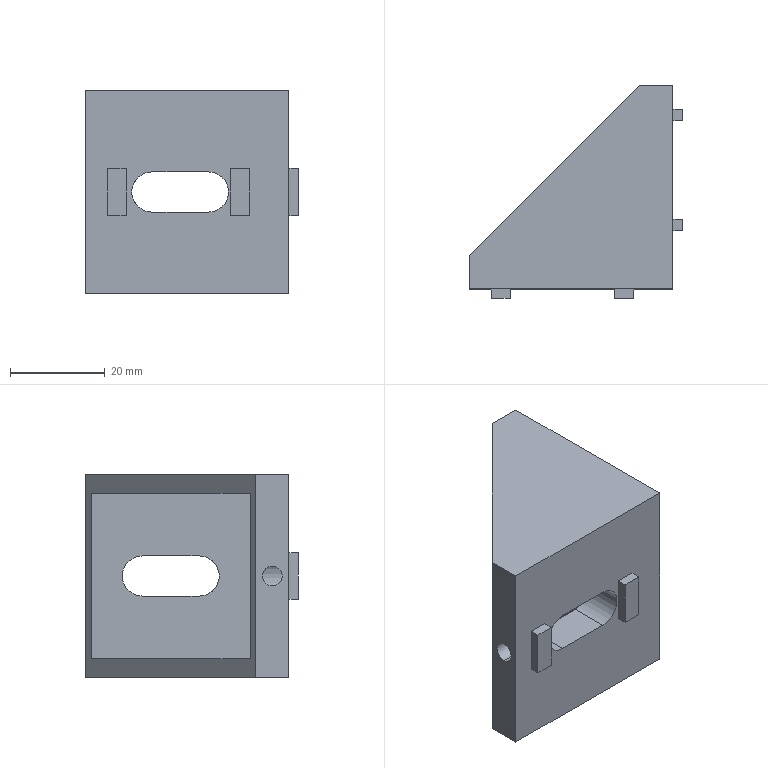Part | STEP file | oyu4545-10_HBLFSND8-45 | 1 solid | 42 faces | box 45 x 45 x 43 mm | volume 29401 mm3 | plane 36 | cylinder 6 | commonest cylinder face diameters 8.5 x4 4.2 x2
STEP:
#1=CARTESIAN_POINT('',(10.305,3.5,-2.1));
#2=VERTEX_POINT('',#1);
#3=CARTESIAN_POINT('',(10.305,3.5,2.1));
#4=VERTEX_POINT('',#3);
#5=CARTESIAN_POINT('',(10.305,3.5,-2.1));
#6=CARTESIAN_POINT('',(10.305,3.361,-2.1));
#7=CARTESIAN_POINT('',(10.297,3.219,-2.086));
#8=CARTESIAN_POINT('',(10.266,2.948,-2.031));
#9=CARTESIAN_POINT('',(10.244,2.816,-1.99));
#10=CARTESIAN_POINT('',(10.19,2.561,-1.883));
#11=CARTESIAN_POINT('',(10.158,2.441,-1.819));
#12=CARTESIAN_POINT('',(10.09,2.216,-1.668));
#13=CARTESIAN_POINT('',(10.053,2.111,-1.58));
#14=CARTESIAN_POINT('',(9.982,1.92,-1.39));
#15=CARTESIAN_POINT('',(9.947,1.834,-1.286));
#16=CARTESIAN_POINT('',(9.883,1.682,-1.06));
#17=CARTESIAN_POINT('',(9.853,1.616,-0.938));
#18=CARTESIAN_POINT('',(9.804,1.51,-0.686));
#19=CARTESIAN_POINT('',(9.784,1.47,-0.5547));
#20=CARTESIAN_POINT('',(9.757,1.414,-0.2804));
#21=CARTESIAN_POINT('',(9.75,1.4,-0.1406));
#22=CARTESIAN_POINT('',(9.75,1.4,0.1373));
#23=CARTESIAN_POINT('',(9.757,1.414,0.2781));
#24=CARTESIAN_POINT('',(9.784,1.469,0.5516));
#25=CARTESIAN_POINT('',(9.803,1.51,0.6835));
#26=CARTESIAN_POINT('',(9.877,1.669,1.065));
#27=CARTESIAN_POINT('',(9.947,1.824,1.294));
#28=CARTESIAN_POINT('',(10.054,2.112,1.582));
#29=CARTESIAN_POINT('',(10.09,2.216,1.667));
#30=CARTESIAN_POINT('',(10.158,2.441,1.818));
#31=CARTESIAN_POINT('',(10.19,2.562,1.884));
#32=CARTESIAN_POINT('',(10.244,2.815,1.99));
#33=CARTESIAN_POINT('',(10.266,2.945,2.03));
#34=CARTESIAN_POINT('',(10.297,3.217,2.085));
#35=CARTESIAN_POINT('',(10.305,3.359,2.1));
#36=CARTESIAN_POINT('',(10.305,3.5,2.1));
#37=B_SPLINE_CURVE_WITH_KNOTS('',3,(#5,#6,#7,#8,#9,#10,#11,#12,#13,#14,#15,#16,#17,#18,#19,#20,#21,#22,#23,#24,#25,#26,#27,#28,#29,#30,#31,#32,#33,#34,#35,#36),.UNSPECIFIED.,.F.,.F.,(4,2,2,2,2,2,2,2,2,2,2,2,2,2,2,4),(0.006676,0.007093,0.007509,0.007926,0.008343,0.008759,0.009176,0.009592,0.01001,0.01043,0.01084,0.01168,0.01209,0.01251,0.01292,0.01334),.UNSPECIFIED.);
#38=EDGE_CURVE('',#2,#4,#37,.T.);
#39=ORIENTED_EDGE('',*,*,#38,.F.);
#40=CARTESIAN_POINT('',(0.,3.5,-2.1));
#41=VERTEX_POINT('',#40);
#42=CARTESIAN_POINT('',(13.,3.5,-2.1));
#43=DIRECTION('',(-1.,0.,0.));
#44=VECTOR('',#43,1000.);
#45=LINE('',#42,#44);
#46=EDGE_CURVE('',#2,#41,#45,.T.);
#47=ORIENTED_EDGE('',*,*,#46,.T.);
#48=CARTESIAN_POINT('',(0.,3.5,2.1));
#49=VERTEX_POINT('',#48);
#50=CARTESIAN_POINT('',(0.,3.5,0.));
#51=DIRECTION('',(1.,0.,0.));
#52=DIRECTION('',(0.,0.,-1.));
#53=AXIS2_PLACEMENT_3D('',#50,#51,#52);
#54=CIRCLE('',#53,2.1);
#55=EDGE_CURVE('',#49,#41,#54,.T.);
#56=ORIENTED_EDGE('',*,*,#55,.F.);
#57=CARTESIAN_POINT('',(13.,3.5,2.1));
#58=DIRECTION('',(-1.,0.,0.));
#59=VECTOR('',#58,1000.);
#60=LINE('',#57,#59);
#61=EDGE_CURVE('',#4,#49,#60,.T.);
#62=ORIENTED_EDGE('',*,*,#61,.F.);
#63=EDGE_LOOP('',(#39,#47,#56,#62));
#64=FACE_OUTER_BOUND('',#63,.T.);
#65=CARTESIAN_POINT('',(13.,3.5,0.));
#66=DIRECTION('',(-1.,0.,0.));
#67=DIRECTION('',(0.,0.,1.));
#68=AXIS2_PLACEMENT_3D('',#65,#66,#67);
#69=CYLINDRICAL_SURFACE('',#68,2.1);
#70=ADVANCED_FACE('',(#64),#69,.F.);
#71=CARTESIAN_POINT('',(43.,38.029,5.));
#72=VERTEX_POINT('',#71);
#73=CARTESIAN_POINT('',(43.,35.599,5.));
#74=VERTEX_POINT('',#73);
#75=CARTESIAN_POINT('',(43.,38.029,5.));
#76=DIRECTION('',(0.,-1.,0.));
#77=VECTOR('',#76,1000.);
#78=LINE('',#75,#77);
#79=EDGE_CURVE('',#72,#74,#78,.T.);
#80=ORIENTED_EDGE('',*,*,#79,.F.);
#81=CARTESIAN_POINT('',(43.,38.029,-5.));
#82=VERTEX_POINT('',#81);
#83=CARTESIAN_POINT('',(43.,38.029,-5.));
#84=DIRECTION('',(0.,0.,1.));
#85=VECTOR('',#84,1000.);
#86=LINE('',#83,#85);
#87=EDGE_CURVE('',#82,#72,#86,.T.);
#88=ORIENTED_EDGE('',*,*,#87,.F.);
#89=CARTESIAN_POINT('',(43.,35.599,-5.));
#90=VERTEX_POINT('',#89);
#91=CARTESIAN_POINT('',(43.,38.029,-5.));
#92=DIRECTION('',(0.,1.,0.));
#93=VECTOR('',#92,1000.);
#94=LINE('',#91,#93);
#95=EDGE_CURVE('',#90,#82,#94,.T.);
#96=ORIENTED_EDGE('',*,*,#95,.F.);
#97=CARTESIAN_POINT('',(43.,35.599,-5.));
#98=DIRECTION('',(0.,0.,-1.));
#99=VECTOR('',#98,1000.);
#100=LINE('',#97,#99);
#101=EDGE_CURVE('',#74,#90,#100,.T.);
#102=ORIENTED_EDGE('',*,*,#101,.F.);
#103=EDGE_LOOP('',(#80,#88,#96,#102));
#104=FACE_BOUND('',#103,.T.);
#105=CARTESIAN_POINT('',(43.,0.,21.5));
#106=VERTEX_POINT('',#105);
#107=CARTESIAN_POINT('',(43.,0.,-21.5));
#108=VERTEX_POINT('',#107);
#109=CARTESIAN_POINT('',(43.,0.,21.5));
#110=DIRECTION('',(0.,0.,-1.));
#111=VECTOR('',#110,1000.);
#112=LINE('',#109,#111);
#113=EDGE_CURVE('',#106,#108,#112,.T.);
#114=ORIENTED_EDGE('',*,*,#113,.T.);
#115=CARTESIAN_POINT('',(43.,43.,-21.5));
#116=VERTEX_POINT('',#115);
#117=CARTESIAN_POINT('',(43.,0.,-21.5));
#118=DIRECTION('',(0.,1.,0.));
#119=VECTOR('',#118,1000.);
#120=LINE('',#117,#119);
#121=EDGE_CURVE('',#108,#116,#120,.T.);
#122=ORIENTED_EDGE('',*,*,#121,.T.);
#123=CARTESIAN_POINT('',(43.,43.,21.5));
#124=VERTEX_POINT('',#123);
#125=CARTESIAN_POINT('',(43.,43.,21.5));
#126=DIRECTION('',(0.,0.,-1.));
#127=VECTOR('',#126,1000.);
#128=LINE('',#125,#127);
#129=EDGE_CURVE('',#124,#116,#128,.T.);
#130=ORIENTED_EDGE('',*,*,#129,.F.);
#131=CARTESIAN_POINT('',(43.,0.,21.5));
#132=DIRECTION('',(0.,1.,0.));
#133=VECTOR('',#132,1000.);
#134=LINE('',#131,#133);
#135=EDGE_CURVE('',#106,#124,#134,.T.);
#136=ORIENTED_EDGE('',*,*,#135,.F.);
#137=EDGE_LOOP('',(#114,#122,#130,#136));
#138=FACE_OUTER_BOUND('',#137,.T.);
#139=CARTESIAN_POINT('',(43.,14.776,-5.));
#140=VERTEX_POINT('',#139);
#141=CARTESIAN_POINT('',(43.,14.776,-0.4688));
#142=VERTEX_POINT('',#141);
#143=CARTESIAN_POINT('',(43.,14.776,5.));
#144=DIRECTION('',(0.,0.,1.));
#145=VECTOR('',#144,1000.);
#146=LINE('',#143,#145);
#147=EDGE_CURVE('',#140,#142,#146,.T.);
#148=ORIENTED_EDGE('',*,*,#147,.F.);
#149=CARTESIAN_POINT('',(43.,12.346,-5.));
#150=VERTEX_POINT('',#149);
#151=CARTESIAN_POINT('',(43.,14.776,-5.));
#152=DIRECTION('',(0.,1.,0.));
#153=VECTOR('',#152,1000.);
#154=LINE('',#151,#153);
#155=EDGE_CURVE('',#150,#140,#154,.T.);
#156=ORIENTED_EDGE('',*,*,#155,.F.);
#157=CARTESIAN_POINT('',(43.,12.346,5.));
#158=VERTEX_POINT('',#157);
#159=CARTESIAN_POINT('',(43.,12.346,5.));
#160=DIRECTION('',(0.,0.,-1.));
#161=VECTOR('',#160,1000.);
#162=LINE('',#159,#161);
#163=EDGE_CURVE('',#158,#150,#162,.T.);
#164=ORIENTED_EDGE('',*,*,#163,.F.);
#165=CARTESIAN_POINT('',(43.,14.776,5.));
#166=VERTEX_POINT('',#165);
#167=CARTESIAN_POINT('',(43.,14.776,5.));
#168=DIRECTION('',(0.,-1.,0.));
#169=VECTOR('',#168,1000.);
#170=LINE('',#167,#169);
#171=EDGE_CURVE('',#166,#158,#170,.T.);
#172=ORIENTED_EDGE('',*,*,#171,.F.);
#173=CARTESIAN_POINT('',(43.,14.776,0.4688));
#174=VERTEX_POINT('',#173);
#175=CARTESIAN_POINT('',(43.,14.776,5.));
#176=DIRECTION('',(0.,0.,1.));
#177=VECTOR('',#176,1000.);
#178=LINE('',#175,#177);
#179=EDGE_CURVE('',#174,#166,#178,.T.);
#180=ORIENTED_EDGE('',*,*,#179,.F.);
#181=CARTESIAN_POINT('',(43.,19.,4.25));
#182=VERTEX_POINT('',#181);
#183=CARTESIAN_POINT('',(43.,19.,0.));
#184=DIRECTION('',(1.,0.,0.));
#185=DIRECTION('',(0.,0.,1.));
#186=AXIS2_PLACEMENT_3D('',#183,#184,#185);
#187=CIRCLE('',#186,4.25);
#188=EDGE_CURVE('',#182,#174,#187,.T.);
#189=ORIENTED_EDGE('',*,*,#188,.F.);
#190=CARTESIAN_POINT('',(43.,31.,4.25));
#191=VERTEX_POINT('',#190);
#192=CARTESIAN_POINT('',(43.,0.,4.25));
#193=DIRECTION('',(0.,-1.,0.));
#194=VECTOR('',#193,1000.);
#195=LINE('',#192,#194);
#196=EDGE_CURVE('',#191,#182,#195,.T.);
#197=ORIENTED_EDGE('',*,*,#196,.F.);
#198=CARTESIAN_POINT('',(43.,31.,-4.25));
#199=VERTEX_POINT('',#198);
#200=CARTESIAN_POINT('',(43.,31.,0.));
#201=DIRECTION('',(1.,0.,0.));
#202=DIRECTION('',(0.,0.,1.));
#203=AXIS2_PLACEMENT_3D('',#200,#201,#202);
#204=CIRCLE('',#203,4.25);
#205=EDGE_CURVE('',#199,#191,#204,.T.);
#206=ORIENTED_EDGE('',*,*,#205,.F.);
#207=CARTESIAN_POINT('',(43.,19.,-4.25));
#208=VERTEX_POINT('',#207);
#209=CARTESIAN_POINT('',(43.,0.,-4.25));
#210=DIRECTION('',(0.,1.,0.));
#211=VECTOR('',#210,1000.);
#212=LINE('',#209,#211);
#213=EDGE_CURVE('',#208,#199,#212,.T.);
#214=ORIENTED_EDGE('',*,*,#213,.F.);
#215=CARTESIAN_POINT('',(43.,19.,0.));
#216=DIRECTION('',(1.,0.,0.));
#217=DIRECTION('',(0.,0.,1.));
#218=AXIS2_PLACEMENT_3D('',#215,#216,#217);
#219=CIRCLE('',#218,4.25);
#220=EDGE_CURVE('',#142,#208,#219,.T.);
#221=ORIENTED_EDGE('',*,*,#220,.F.);
#222=EDGE_LOOP('',(#148,#156,#164,#172,#180,#189,#197,#206,#214,#221));
#223=FACE_BOUND('',#222,.T.);
#224=CARTESIAN_POINT('',(43.,0.,21.5));
#225=DIRECTION('',(-1.,0.,0.));
#226=DIRECTION('',(0.,0.,1.));
#227=AXIS2_PLACEMENT_3D('',#224,#225,#226);
#228=PLANE('',#227);
#229=ADVANCED_FACE('',(#104,#138,#223),#228,.F.);
#230=CARTESIAN_POINT('',(0.,7.,21.5));
#231=VERTEX_POINT('',#230);
#232=CARTESIAN_POINT('',(0.,0.,21.5));
#233=VERTEX_POINT('',#232);
#234=CARTESIAN_POINT('',(0.,43.,21.5));
#235=DIRECTION('',(0.,-1.,0.));
#236=VECTOR('',#235,1000.);
#237=LINE('',#234,#236);
#238=EDGE_CURVE('',#231,#233,#237,.T.);
#239=ORIENTED_EDGE('',*,*,#238,.F.);
#240=CARTESIAN_POINT('',(0.,7.,-21.5));
#241=VERTEX_POINT('',#240);
#242=CARTESIAN_POINT('',(0.,7.,-21.5));
#243=DIRECTION('',(0.,0.,1.));
#244=VECTOR('',#243,1000.);
#245=LINE('',#242,#244);
#246=EDGE_CURVE('',#241,#231,#245,.T.);
#247=ORIENTED_EDGE('',*,*,#246,.F.);
#248=CARTESIAN_POINT('',(0.,0.,-21.5));
#249=VERTEX_POINT('',#248);
#250=CARTESIAN_POINT('',(0.,43.,-21.5));
#251=DIRECTION('',(0.,-1.,0.));
#252=VECTOR('',#251,1000.);
#253=LINE('',#250,#252);
#254=EDGE_CURVE('',#241,#249,#253,.T.);
#255=ORIENTED_EDGE('',*,*,#254,.T.);
#256=CARTESIAN_POINT('',(0.,0.,21.5));
#257=DIRECTION('',(0.,0.,-1.));
#258=VECTOR('',#257,1000.);
#259=LINE('',#256,#258);
#260=EDGE_CURVE('',#233,#249,#259,.T.);
#261=ORIENTED_EDGE('',*,*,#260,.F.);
#262=EDGE_LOOP('',(#239,#247,#255,#261));
#263=FACE_OUTER_BOUND('',#262,.T.);
#264=ORIENTED_EDGE('',*,*,#55,.T.);
#265=CARTESIAN_POINT('',(0.,3.5,0.));
#266=DIRECTION('',(1.,0.,0.));
#267=DIRECTION('',(0.,0.,-1.));
#268=AXIS2_PLACEMENT_3D('',#265,#266,#267);
#269=CIRCLE('',#268,2.1);
#270=EDGE_CURVE('',#41,#49,#269,.T.);
#271=ORIENTED_EDGE('',*,*,#270,.T.);
#272=EDGE_LOOP('',(#264,#271));
#273=FACE_BOUND('',#272,.T.);
#274=CARTESIAN_POINT('',(0.,43.,21.5));
#275=DIRECTION('',(1.,0.,0.));
#276=DIRECTION('',(0.,0.,-1.));
#277=AXIS2_PLACEMENT_3D('',#274,#275,#276);
#278=PLANE('',#277);
#279=ADVANCED_FACE('',(#263,#273),#278,.F.);
#280=CARTESIAN_POINT('',(14.,8.2,4.25));
#281=VERTEX_POINT('',#280);
#282=CARTESIAN_POINT('',(14.,0.,4.25));
#283=VERTEX_POINT('',#282);
#284=CARTESIAN_POINT('',(14.,43.,4.25));
#285=DIRECTION('',(0.,-1.,0.));
#286=VECTOR('',#285,1000.);
#287=LINE('',#284,#286);
#288=EDGE_CURVE('',#281,#283,#287,.T.);
#289=ORIENTED_EDGE('',*,*,#288,.T.);
#290=CARTESIAN_POINT('',(14.,0.,-4.25));
#291=VERTEX_POINT('',#290);
#292=CARTESIAN_POINT('',(14.,0.,0.));
#293=DIRECTION('',(0.,1.,0.));
#294=DIRECTION('',(0.,0.,1.));
#295=AXIS2_PLACEMENT_3D('',#292,#293,#294);
#296=CIRCLE('',#295,4.25);
#297=EDGE_CURVE('',#291,#283,#296,.T.);
#298=ORIENTED_EDGE('',*,*,#297,.F.);
#299=CARTESIAN_POINT('',(14.,8.2,-4.25));
#300=VERTEX_POINT('',#299);
#301=CARTESIAN_POINT('',(14.,43.,-4.25));
#302=DIRECTION('',(0.,-1.,0.));
#303=VECTOR('',#302,1000.);
#304=LINE('',#301,#303);
#305=EDGE_CURVE('',#300,#291,#304,.T.);
#306=ORIENTED_EDGE('',*,*,#305,.F.);
#307=CARTESIAN_POINT('',(14.,8.2,0.));
#308=DIRECTION('',(0.,-1.,0.));
#309=DIRECTION('',(0.,0.,1.));
#310=AXIS2_PLACEMENT_3D('',#307,#308,#309);
#311=CIRCLE('',#310,4.25);
#312=EDGE_CURVE('',#281,#300,#311,.T.);
#313=ORIENTED_EDGE('',*,*,#312,.F.);
#314=EDGE_LOOP('',(#289,#298,#306,#313));
#315=FACE_OUTER_BOUND('',#314,.T.);
#316=CARTESIAN_POINT('',(10.305,3.5,2.1));
#317=CARTESIAN_POINT('',(10.305,3.641,2.1));
#318=CARTESIAN_POINT('',(10.297,3.78,2.086));
#319=CARTESIAN_POINT('',(10.267,4.051,2.031));
#320=CARTESIAN_POINT('',(10.244,4.185,1.99));
#321=CARTESIAN_POINT('',(10.163,4.565,1.831));
#322=CARTESIAN_POINT('',(10.089,4.794,1.676));
#323=CARTESIAN_POINT('',(9.947,5.175,1.295));
#324=CARTESIAN_POINT('',(9.878,5.331,1.065));
#325=CARTESIAN_POINT('',(9.804,5.489,0.6864));
#326=CARTESIAN_POINT('',(9.784,5.531,0.5517));
#327=CARTESIAN_POINT('',(9.757,5.586,0.2792));
#328=CARTESIAN_POINT('',(9.75,5.6,0.1412));
#329=CARTESIAN_POINT('',(9.75,5.6,-0.1385));
#330=CARTESIAN_POINT('',(9.757,5.586,-0.2799));
#331=CARTESIAN_POINT('',(9.784,5.531,-0.5518));
#332=CARTESIAN_POINT('',(9.804,5.49,-0.6853));
#333=CARTESIAN_POINT('',(9.853,5.383,-0.9404));
#334=CARTESIAN_POINT('',(9.883,5.318,-1.06));
#335=CARTESIAN_POINT('',(9.948,5.166,-1.286));
#336=CARTESIAN_POINT('',(9.983,5.078,-1.392));
#337=CARTESIAN_POINT('',(10.09,4.792,-1.678));
#338=CARTESIAN_POINT('',(10.163,4.561,-1.832));
#339=CARTESIAN_POINT('',(10.244,4.184,-1.99));
#340=CARTESIAN_POINT('',(10.267,4.052,-2.031));
#341=CARTESIAN_POINT('',(10.297,3.777,-2.086));
#342=CARTESIAN_POINT('',(10.305,3.639,-2.1));
#343=CARTESIAN_POINT('',(10.305,3.5,-2.1));
#344=B_SPLINE_CURVE_WITH_KNOTS('',3,(#316,#317,#318,#319,#320,#321,#322,#323,#324,#325,#326,#327,#328,#329,#330,#331,#332,#333,#334,#335,#336,#337,#338,#339,#340,#341,#342,#343),.UNSPECIFIED.,.F.,.F.,(4,2,2,2,2,2,2,2,2,2,2,2,2,4),(0.,0.0004173,0.0008345,0.001669,0.002504,0.002921,0.003338,0.003755,0.004173,0.00459,0.005007,0.005842,0.006259,0.006676),.UNSPECIFIED.);
#345=EDGE_CURVE('',#4,#2,#344,.T.);
#346=ORIENTED_EDGE('',*,*,#345,.T.);
#347=ORIENTED_EDGE('',*,*,#38,.T.);
#348=EDGE_LOOP('',(#346,#347));
#349=FACE_BOUND('',#348,.T.);
#350=CARTESIAN_POINT('',(14.,43.,0.));
#351=DIRECTION('',(0.,-1.,0.));
#352=DIRECTION('',(0.,0.,-1.));
#353=AXIS2_PLACEMENT_3D('',#350,#351,#352);
#354=CYLINDRICAL_SURFACE('',#353,4.25);
#355=ADVANCED_FACE('',(#315,#349),#354,.F.);
#356=CARTESIAN_POINT('',(34.8,8.2,17.5));
#357=VERTEX_POINT('',#356);
#358=CARTESIAN_POINT('',(34.8,41.8,17.5));
#359=VERTEX_POINT('',#358);
#360=CARTESIAN_POINT('',(34.8,8.2,17.5));
#361=DIRECTION('',(0.,1.,0.));
#362=VECTOR('',#361,1000.);
#363=LINE('',#360,#362);
#364=EDGE_CURVE('',#357,#359,#363,.T.);
#365=ORIENTED_EDGE('',*,*,#364,.T.);
#366=CARTESIAN_POINT('',(34.8,41.8,-17.5));
#367=VERTEX_POINT('',#366);
#368=CARTESIAN_POINT('',(34.8,41.8,17.5));
#369=DIRECTION('',(0.,0.,-1.));
#370=VECTOR('',#369,1000.);
#371=LINE('',#368,#370);
#372=EDGE_CURVE('',#359,#367,#371,.T.);
#373=ORIENTED_EDGE('',*,*,#372,.T.);
#374=CARTESIAN_POINT('',(34.8,8.2,-17.5));
#375=VERTEX_POINT('',#374);
#376=CARTESIAN_POINT('',(34.8,8.2,-17.5));
#377=DIRECTION('',(0.,1.,0.));
#378=VECTOR('',#377,1000.);
#379=LINE('',#376,#378);
#380=EDGE_CURVE('',#375,#367,#379,.T.);
#381=ORIENTED_EDGE('',*,*,#380,.F.);
#382=CARTESIAN_POINT('',(34.8,8.2,17.5));
#383=DIRECTION('',(0.,0.,-1.));
#384=VECTOR('',#383,1000.);
#385=LINE('',#382,#384);
#386=EDGE_CURVE('',#357,#375,#385,.T.);
#387=ORIENTED_EDGE('',*,*,#386,.F.);
#388=EDGE_LOOP('',(#365,#373,#381,#387));
#389=FACE_OUTER_BOUND('',#388,.T.);
#390=CARTESIAN_POINT('',(34.8,19.,-4.25));
#391=VERTEX_POINT('',#390);
#392=CARTESIAN_POINT('',(34.8,19.,4.25));
#393=VERTEX_POINT('',#392);
#394=CARTESIAN_POINT('',(34.8,19.,0.));
#395=DIRECTION('',(-1.,0.,0.));
#396=DIRECTION('',(0.,0.,-1.));
#397=AXIS2_PLACEMENT_3D('',#394,#395,#396);
#398=CIRCLE('',#397,4.25);
#399=EDGE_CURVE('',#391,#393,#398,.T.);
#400=ORIENTED_EDGE('',*,*,#399,.F.);
#401=CARTESIAN_POINT('',(34.8,31.,-4.25));
#402=VERTEX_POINT('',#401);
#403=CARTESIAN_POINT('',(34.8,8.2,-4.25));
#404=DIRECTION('',(0.,-1.,0.));
#405=VECTOR('',#404,1000.);
#406=LINE('',#403,#405);
#407=EDGE_CURVE('',#402,#391,#406,.T.);
#408=ORIENTED_EDGE('',*,*,#407,.F.);
#409=CARTESIAN_POINT('',(34.8,31.,4.25));
#410=VERTEX_POINT('',#409);
#411=CARTESIAN_POINT('',(34.8,31.,0.));
#412=DIRECTION('',(-1.,0.,0.));
#413=DIRECTION('',(0.,0.,-1.));
#414=AXIS2_PLACEMENT_3D('',#411,#412,#413);
#415=CIRCLE('',#414,4.25);
#416=EDGE_CURVE('',#410,#402,#415,.T.);
#417=ORIENTED_EDGE('',*,*,#416,.F.);
#418=CARTESIAN_POINT('',(34.8,8.2,4.25));
#419=DIRECTION('',(0.,1.,0.));
#420=VECTOR('',#419,1000.);
#421=LINE('',#418,#420);
#422=EDGE_CURVE('',#393,#410,#421,.T.);
#423=ORIENTED_EDGE('',*,*,#422,.F.);
#424=EDGE_LOOP('',(#400,#408,#417,#423));
#425=FACE_BOUND('',#424,.T.);
#426=CARTESIAN_POINT('',(34.8,8.2,17.5));
#427=DIRECTION('',(1.,0.,0.));
#428=DIRECTION('',(0.,0.,-1.));
#429=AXIS2_PLACEMENT_3D('',#426,#427,#428);
#430=PLANE('',#429);
#431=ADVANCED_FACE('',(#389,#425),#430,.F.);
#432=ORIENTED_EDGE('',*,*,#260,.T.);
#433=CARTESIAN_POINT('',(0.,0.,-21.5));
#434=DIRECTION('',(1.,0.,0.));
#435=VECTOR('',#434,1000.);
#436=LINE('',#433,#435);
#437=EDGE_CURVE('',#249,#108,#436,.T.);
#438=ORIENTED_EDGE('',*,*,#437,.T.);
#439=ORIENTED_EDGE('',*,*,#113,.F.);
#440=CARTESIAN_POINT('',(0.,0.,21.5));
#441=DIRECTION('',(1.,0.,0.));
#442=VECTOR('',#441,1000.);
#443=LINE('',#440,#442);
#444=EDGE_CURVE('',#233,#106,#443,.T.);
#445=ORIENTED_EDGE('',*,*,#444,.F.);
#446=EDGE_LOOP('',(#432,#438,#439,#445));
#447=FACE_OUTER_BOUND('',#446,.T.);
#448=CARTESIAN_POINT('',(4.6,0.,4.9));
#449=VERTEX_POINT('',#448);
#450=CARTESIAN_POINT('',(4.6,0.,-4.9));
#451=VERTEX_POINT('',#450);
#452=CARTESIAN_POINT('',(4.6,0.,4.9));
#453=DIRECTION('',(0.,0.,-1.));
#454=VECTOR('',#453,1000.);
#455=LINE('',#452,#454);
#456=EDGE_CURVE('',#449,#451,#455,.T.);
#457=ORIENTED_EDGE('',*,*,#456,.F.);
#458=CARTESIAN_POINT('',(8.6,0.,4.9));
#459=VERTEX_POINT('',#458);
#460=CARTESIAN_POINT('',(8.6,0.,4.9));
#461=DIRECTION('',(-1.,0.,0.));
#462=VECTOR('',#461,1000.);
#463=LINE('',#460,#462);
#464=EDGE_CURVE('',#459,#449,#463,.T.);
#465=ORIENTED_EDGE('',*,*,#464,.F.);
#466=CARTESIAN_POINT('',(8.6,0.,-4.9));
#467=VERTEX_POINT('',#466);
#468=CARTESIAN_POINT('',(8.6,0.,4.9));
#469=DIRECTION('',(0.,0.,-1.));
#470=VECTOR('',#469,1000.);
#471=LINE('',#468,#470);
#472=EDGE_CURVE('',#459,#467,#471,.T.);
#473=ORIENTED_EDGE('',*,*,#472,.T.);
#474=CARTESIAN_POINT('',(8.6,0.,-4.9));
#475=DIRECTION('',(-1.,0.,0.));
#476=VECTOR('',#475,1000.);
#477=LINE('',#474,#476);
#478=EDGE_CURVE('',#467,#451,#477,.T.);
#479=ORIENTED_EDGE('',*,*,#478,.T.);
#480=EDGE_LOOP('',(#457,#465,#473,#479));
#481=FACE_BOUND('',#480,.T.);
#482=CARTESIAN_POINT('',(30.682,0.,4.9));
#483=VERTEX_POINT('',#482);
#484=CARTESIAN_POINT('',(30.682,0.,-4.9));
#485=VERTEX_POINT('',#484);
#486=CARTESIAN_POINT('',(30.682,0.,4.9));
#487=DIRECTION('',(0.,0.,-1.));
#488=VECTOR('',#487,1000.);
#489=LINE('',#486,#488);
#490=EDGE_CURVE('',#483,#485,#489,.T.);
#491=ORIENTED_EDGE('',*,*,#490,.F.);
#492=CARTESIAN_POINT('',(34.72,0.,4.9));
#493=VERTEX_POINT('',#492);
#494=CARTESIAN_POINT('',(34.72,0.,4.9));
#495=DIRECTION('',(-1.,0.,0.));
#496=VECTOR('',#495,1000.);
#497=LINE('',#494,#496);
#498=EDGE_CURVE('',#493,#483,#497,.T.);
#499=ORIENTED_EDGE('',*,*,#498,.F.);
#500=CARTESIAN_POINT('',(34.72,0.,-4.9));
#501=VERTEX_POINT('',#500);
#502=CARTESIAN_POINT('',(34.72,0.,4.9));
#503=DIRECTION('',(0.,0.,-1.));
#504=VECTOR('',#503,1000.);
#505=LINE('',#502,#504);
#506=EDGE_CURVE('',#493,#501,#505,.T.);
#507=ORIENTED_EDGE('',*,*,#506,.T.);
#508=CARTESIAN_POINT('',(34.72,0.,-4.9));
#509=DIRECTION('',(-1.,0.,0.));
#510=VECTOR('',#509,1000.);
#511=LINE('',#508,#510);
#512=EDGE_CURVE('',#501,#485,#511,.T.);
#513=ORIENTED_EDGE('',*,*,#512,.T.);
#514=EDGE_LOOP('',(#491,#499,#507,#513));
#515=FACE_BOUND('',#514,.T.);
#516=ORIENTED_EDGE('',*,*,#297,.T.);
#517=CARTESIAN_POINT('',(26.,0.,4.25));
#518=VERTEX_POINT('',#517);
#519=CARTESIAN_POINT('',(14.,0.,4.25));
#520=DIRECTION('',(1.,0.,0.));
#521=VECTOR('',#520,1000.);
#522=LINE('',#519,#521);
#523=EDGE_CURVE('',#283,#518,#522,.T.);
#524=ORIENTED_EDGE('',*,*,#523,.T.);
#525=CARTESIAN_POINT('',(26.,0.,-4.25));
#526=VERTEX_POINT('',#525);
#527=CARTESIAN_POINT('',(26.,0.,0.));
#528=DIRECTION('',(0.,1.,0.));
#529=DIRECTION('',(0.,0.,1.));
#530=AXIS2_PLACEMENT_3D('',#527,#528,#529);
#531=CIRCLE('',#530,4.25);
#532=EDGE_CURVE('',#518,#526,#531,.T.);
#533=ORIENTED_EDGE('',*,*,#532,.T.);
#534=CARTESIAN_POINT('',(14.,0.,-4.25));
#535=DIRECTION('',(-1.,0.,0.));
#536=VECTOR('',#535,1000.);
#537=LINE('',#534,#536);
#538=EDGE_CURVE('',#526,#291,#537,.T.);
#539=ORIENTED_EDGE('',*,*,#538,.T.);
#540=EDGE_LOOP('',(#516,#524,#533,#539));
#541=FACE_BOUND('',#540,.T.);
#542=CARTESIAN_POINT('',(0.,0.,21.5));
#543=DIRECTION('',(0.,1.,0.));
#544=DIRECTION('',(0.,0.,1.));
#545=AXIS2_PLACEMENT_3D('',#542,#543,#544);
#546=PLANE('',#545);
#547=ADVANCED_FACE('',(#447,#481,#515,#541),#546,.F.);
#548=CARTESIAN_POINT('',(1.2,8.2,17.5));
#549=VERTEX_POINT('',#548);
#550=CARTESIAN_POINT('',(1.2,8.2,-17.5));
#551=VERTEX_POINT('',#550);
#552=CARTESIAN_POINT('',(1.2,8.2,-17.5));
#553=DIRECTION('',(0.,0.,-1.));
#554=VECTOR('',#553,1000.);
#555=LINE('',#552,#554);
#556=EDGE_CURVE('',#549,#551,#555,.T.);
#557=ORIENTED_EDGE('',*,*,#556,.F.);
#558=CARTESIAN_POINT('',(0.,8.2,17.5));
#559=DIRECTION('',(1.,0.,0.));
#560=VECTOR('',#559,1000.);
#561=LINE('',#558,#560);
#562=EDGE_CURVE('',#549,#357,#561,.T.);
#563=ORIENTED_EDGE('',*,*,#562,.T.);
#564=ORIENTED_EDGE('',*,*,#386,.T.);
#565=CARTESIAN_POINT('',(34.8,8.2,-17.5));
#566=DIRECTION('',(-1.,0.,0.));
#567=VECTOR('',#566,1000.);
#568=LINE('',#565,#567);
#569=EDGE_CURVE('',#375,#551,#568,.T.);
#570=ORIENTED_EDGE('',*,*,#569,.T.);
#571=EDGE_LOOP('',(#557,#563,#564,#570));
#572=FACE_OUTER_BOUND('',#571,.T.);
#573=CARTESIAN_POINT('',(26.,8.2,4.25));
#574=VERTEX_POINT('',#573);
#575=CARTESIAN_POINT('',(0.,8.2,4.25));
#576=DIRECTION('',(-1.,0.,0.));
#577=VECTOR('',#576,1000.);
#578=LINE('',#575,#577);
#579=EDGE_CURVE('',#574,#281,#578,.T.);
#580=ORIENTED_EDGE('',*,*,#579,.T.);
#581=ORIENTED_EDGE('',*,*,#312,.T.);
#582=CARTESIAN_POINT('',(26.,8.2,-4.25));
#583=VERTEX_POINT('',#582);
#584=CARTESIAN_POINT('',(0.,8.2,-4.25));
#585=DIRECTION('',(1.,0.,0.));
#586=VECTOR('',#585,1000.);
#587=LINE('',#584,#586);
#588=EDGE_CURVE('',#300,#583,#587,.T.);
#589=ORIENTED_EDGE('',*,*,#588,.T.);
#590=CARTESIAN_POINT('',(26.,8.2,0.));
#591=DIRECTION('',(0.,-1.,0.));
#592=DIRECTION('',(0.,0.,1.));
#593=AXIS2_PLACEMENT_3D('',#590,#591,#592);
#594=CIRCLE('',#593,4.25);
#595=EDGE_CURVE('',#583,#574,#594,.T.);
#596=ORIENTED_EDGE('',*,*,#595,.T.);
#597=EDGE_LOOP('',(#580,#581,#589,#596));
#598=FACE_BOUND('',#597,.T.);
#599=CARTESIAN_POINT('',(0.,8.2,-17.5));
#600=DIRECTION('',(0.,1.,0.));
#601=DIRECTION('',(0.,0.,1.));
#602=AXIS2_PLACEMENT_3D('',#599,#600,#601);
#603=PLANE('',#602);
#604=ADVANCED_FACE('',(#572,#598),#603,.T.);
#605=CARTESIAN_POINT('',(36.,43.,-21.5));
#606=VERTEX_POINT('',#605);
#607=CARTESIAN_POINT('',(43.,43.,-21.5));
#608=DIRECTION('',(-1.,0.,0.));
#609=VECTOR('',#608,1000.);
#610=LINE('',#607,#609);
#611=EDGE_CURVE('',#116,#606,#610,.T.);
#612=ORIENTED_EDGE('',*,*,#611,.T.);
#613=CARTESIAN_POINT('',(36.,43.,21.5));
#614=VERTEX_POINT('',#613);
#615=CARTESIAN_POINT('',(36.,43.,-21.5));
#616=DIRECTION('',(0.,0.,1.));
#617=VECTOR('',#616,1000.);
#618=LINE('',#615,#617);
#619=EDGE_CURVE('',#606,#614,#618,.T.);
#620=ORIENTED_EDGE('',*,*,#619,.T.);
#621=CARTESIAN_POINT('',(43.,43.,21.5));
#622=DIRECTION('',(-1.,0.,0.));
#623=VECTOR('',#622,1000.);
#624=LINE('',#621,#623);
#625=EDGE_CURVE('',#124,#614,#624,.T.);
#626=ORIENTED_EDGE('',*,*,#625,.F.);
#627=ORIENTED_EDGE('',*,*,#129,.T.);
#628=EDGE_LOOP('',(#612,#620,#626,#627));
#629=FACE_OUTER_BOUND('',#628,.T.);
#630=CARTESIAN_POINT('',(43.,43.,21.5));
#631=DIRECTION('',(0.,-1.,0.));
#632=DIRECTION('',(0.,0.,-1.));
#633=AXIS2_PLACEMENT_3D('',#630,#631,#632);
#634=PLANE('',#633);
#635=ADVANCED_FACE('',(#629),#634,.F.);
#636=CARTESIAN_POINT('',(0.,7.,21.5));
#637=DIRECTION('',(0.7071,0.7071,0.));
#638=VECTOR('',#637,1000.);
#639=LINE('',#636,#638);
#640=EDGE_CURVE('',#231,#614,#639,.T.);
#641=ORIENTED_EDGE('',*,*,#640,.F.);
#642=ORIENTED_EDGE('',*,*,#238,.T.);
#643=ORIENTED_EDGE('',*,*,#444,.T.);
#644=ORIENTED_EDGE('',*,*,#135,.T.);
#645=ORIENTED_EDGE('',*,*,#625,.T.);
#646=EDGE_LOOP('',(#641,#642,#643,#644,#645));
#647=FACE_OUTER_BOUND('',#646,.T.);
#648=CARTESIAN_POINT('',(0.,0.,21.5));
#649=DIRECTION('',(0.,0.,1.));
#650=DIRECTION('',(1.,0.,0.));
#651=AXIS2_PLACEMENT_3D('',#648,#649,#650);
#652=PLANE('',#651);
#653=ADVANCED_FACE('',(#647),#652,.T.);
#654=ORIENTED_EDGE('',*,*,#254,.F.);
#655=CARTESIAN_POINT('',(0.,7.,-21.5));
#656=DIRECTION('',(0.7071,0.7071,0.));
#657=VECTOR('',#656,1000.);
#658=LINE('',#655,#657);
#659=EDGE_CURVE('',#241,#606,#658,.T.);
#660=ORIENTED_EDGE('',*,*,#659,.T.);
#661=ORIENTED_EDGE('',*,*,#611,.F.);
#662=ORIENTED_EDGE('',*,*,#121,.F.);
#663=ORIENTED_EDGE('',*,*,#437,.F.);
#664=EDGE_LOOP('',(#654,#660,#661,#662,#663));
#665=FACE_OUTER_BOUND('',#664,.T.);
#666=CARTESIAN_POINT('',(0.,0.,-21.5));
#667=DIRECTION('',(0.,0.,1.));
#668=DIRECTION('',(1.,0.,0.));
#669=AXIS2_PLACEMENT_3D('',#666,#667,#668);
#670=PLANE('',#669);
#671=ADVANCED_FACE('',(#665),#670,.F.);
#672=ORIENTED_EDGE('',*,*,#380,.T.);
#673=CARTESIAN_POINT('',(18.,25.,-17.5));
#674=DIRECTION('',(-0.7071,-0.7071,0.));
#675=VECTOR('',#674,1000.);
#676=LINE('',#673,#675);
#677=EDGE_CURVE('',#367,#551,#676,.T.);
#678=ORIENTED_EDGE('',*,*,#677,.T.);
#679=ORIENTED_EDGE('',*,*,#569,.F.);
#680=EDGE_LOOP('',(#672,#678,#679));
#681=FACE_OUTER_BOUND('',#680,.T.);
#682=CARTESIAN_POINT('',(34.8,8.2,-17.5));
#683=DIRECTION('',(0.,0.,-1.));
#684=DIRECTION('',(-1.,0.,0.));
#685=AXIS2_PLACEMENT_3D('',#682,#683,#684);
#686=PLANE('',#685);
#687=ADVANCED_FACE('',(#681),#686,.F.);
#688=ORIENTED_EDGE('',*,*,#562,.F.);
#689=CARTESIAN_POINT('',(0.6,7.6,17.5));
#690=DIRECTION('',(0.7071,0.7071,0.));
#691=VECTOR('',#690,1000.);
#692=LINE('',#689,#691);
#693=EDGE_CURVE('',#549,#359,#692,.T.);
#694=ORIENTED_EDGE('',*,*,#693,.T.);
#695=ORIENTED_EDGE('',*,*,#364,.F.);
#696=EDGE_LOOP('',(#688,#694,#695));
#697=FACE_OUTER_BOUND('',#696,.T.);
#698=CARTESIAN_POINT('',(0.,8.2,17.5));
#699=DIRECTION('',(0.,0.,1.));
#700=DIRECTION('',(1.,0.,0.));
#701=AXIS2_PLACEMENT_3D('',#698,#699,#700);
#702=PLANE('',#701);
#703=ADVANCED_FACE('',(#697),#702,.F.);
#704=ORIENTED_EDGE('',*,*,#456,.T.);
#705=CARTESIAN_POINT('',(4.6,-2.,-4.9));
#706=VERTEX_POINT('',#705);
#707=CARTESIAN_POINT('',(4.6,0.,-4.9));
#708=DIRECTION('',(0.,-1.,0.));
#709=VECTOR('',#708,1000.);
#710=LINE('',#707,#709);
#711=EDGE_CURVE('',#451,#706,#710,.T.);
#712=ORIENTED_EDGE('',*,*,#711,.T.);
#713=CARTESIAN_POINT('',(4.6,-2.,4.9));
#714=VERTEX_POINT('',#713);
#715=CARTESIAN_POINT('',(4.6,-2.,4.9));
#716=DIRECTION('',(0.,0.,-1.));
#717=VECTOR('',#716,1000.);
#718=LINE('',#715,#717);
#719=EDGE_CURVE('',#714,#706,#718,.T.);
#720=ORIENTED_EDGE('',*,*,#719,.F.);
#721=CARTESIAN_POINT('',(4.6,0.,4.9));
#722=DIRECTION('',(0.,-1.,0.));
#723=VECTOR('',#722,1000.);
#724=LINE('',#721,#723);
#725=EDGE_CURVE('',#449,#714,#724,.T.);
#726=ORIENTED_EDGE('',*,*,#725,.F.);
#727=EDGE_LOOP('',(#704,#712,#720,#726));
#728=FACE_OUTER_BOUND('',#727,.T.);
#729=CARTESIAN_POINT('',(4.6,0.,4.9));
#730=DIRECTION('',(1.,0.,0.));
#731=DIRECTION('',(0.,0.,-1.));
#732=AXIS2_PLACEMENT_3D('',#729,#730,#731);
#733=PLANE('',#732);
#734=ADVANCED_FACE('',(#728),#733,.F.);
#735=ORIENTED_EDGE('',*,*,#719,.T.);
#736=CARTESIAN_POINT('',(8.6,-2.,-4.9));
#737=VERTEX_POINT('',#736);
#738=CARTESIAN_POINT('',(4.6,-2.,-4.9));
#739=DIRECTION('',(1.,0.,0.));
#740=VECTOR('',#739,1000.);
#741=LINE('',#738,#740);
#742=EDGE_CURVE('',#706,#737,#741,.T.);
#743=ORIENTED_EDGE('',*,*,#742,.T.);
#744=CARTESIAN_POINT('',(8.6,-2.,4.9));
#745=VERTEX_POINT('',#744);
#746=CARTESIAN_POINT('',(8.6,-2.,4.9));
#747=DIRECTION('',(0.,0.,-1.));
#748=VECTOR('',#747,1000.);
#749=LINE('',#746,#748);
#750=EDGE_CURVE('',#745,#737,#749,.T.);
#751=ORIENTED_EDGE('',*,*,#750,.F.);
#752=CARTESIAN_POINT('',(4.6,-2.,4.9));
#753=DIRECTION('',(1.,0.,0.));
#754=VECTOR('',#753,1000.);
#755=LINE('',#752,#754);
#756=EDGE_CURVE('',#714,#745,#755,.T.);
#757=ORIENTED_EDGE('',*,*,#756,.F.);
#758=EDGE_LOOP('',(#735,#743,#751,#757));
#759=FACE_OUTER_BOUND('',#758,.T.);
#760=CARTESIAN_POINT('',(4.6,-2.,4.9));
#761=DIRECTION('',(0.,1.,0.));
#762=DIRECTION('',(0.,0.,1.));
#763=AXIS2_PLACEMENT_3D('',#760,#761,#762);
#764=PLANE('',#763);
#765=ADVANCED_FACE('',(#759),#764,.F.);
#766=ORIENTED_EDGE('',*,*,#750,.T.);
#767=CARTESIAN_POINT('',(8.6,-2.,-4.9));
#768=DIRECTION('',(0.,1.,0.));
#769=VECTOR('',#768,1000.);
#770=LINE('',#767,#769);
#771=EDGE_CURVE('',#737,#467,#770,.T.);
#772=ORIENTED_EDGE('',*,*,#771,.T.);
#773=ORIENTED_EDGE('',*,*,#472,.F.);
#774=CARTESIAN_POINT('',(8.6,-2.,4.9));
#775=DIRECTION('',(0.,1.,0.));
#776=VECTOR('',#775,1000.);
#777=LINE('',#774,#776);
#778=EDGE_CURVE('',#745,#459,#777,.T.);
#779=ORIENTED_EDGE('',*,*,#778,.F.);
#780=EDGE_LOOP('',(#766,#772,#773,#779));
#781=FACE_OUTER_BOUND('',#780,.T.);
#782=CARTESIAN_POINT('',(8.6,-2.,4.9));
#783=DIRECTION('',(-1.,0.,0.));
#784=DIRECTION('',(0.,0.,1.));
#785=AXIS2_PLACEMENT_3D('',#782,#783,#784);
#786=PLANE('',#785);
#787=ADVANCED_FACE('',(#781),#786,.F.);
#788=ORIENTED_EDGE('',*,*,#464,.T.);
#789=ORIENTED_EDGE('',*,*,#725,.T.);
#790=ORIENTED_EDGE('',*,*,#756,.T.);
#791=ORIENTED_EDGE('',*,*,#778,.T.);
#792=EDGE_LOOP('',(#788,#789,#790,#791));
#793=FACE_OUTER_BOUND('',#792,.T.);
#794=CARTESIAN_POINT('',(4.6,0.,4.9));
#795=DIRECTION('',(0.,0.,1.));
#796=DIRECTION('',(1.,0.,0.));
#797=AXIS2_PLACEMENT_3D('',#794,#795,#796);
#798=PLANE('',#797);
#799=ADVANCED_FACE('',(#793),#798,.T.);
#800=ORIENTED_EDGE('',*,*,#478,.F.);
#801=ORIENTED_EDGE('',*,*,#771,.F.);
#802=ORIENTED_EDGE('',*,*,#742,.F.);
#803=ORIENTED_EDGE('',*,*,#711,.F.);
#804=EDGE_LOOP('',(#800,#801,#802,#803));
#805=FACE_OUTER_BOUND('',#804,.T.);
#806=CARTESIAN_POINT('',(4.6,0.,-4.9));
#807=DIRECTION('',(0.,0.,1.));
#808=DIRECTION('',(1.,0.,0.));
#809=AXIS2_PLACEMENT_3D('',#806,#807,#808);
#810=PLANE('',#809);
#811=ADVANCED_FACE('',(#805),#810,.F.);
#812=ORIENTED_EDGE('',*,*,#490,.T.);
#813=CARTESIAN_POINT('',(30.682,-2.,-4.9));
#814=VERTEX_POINT('',#813);
#815=CARTESIAN_POINT('',(30.682,0.,-4.9));
#816=DIRECTION('',(0.,-1.,0.));
#817=VECTOR('',#816,1000.);
#818=LINE('',#815,#817);
#819=EDGE_CURVE('',#485,#814,#818,.T.);
#820=ORIENTED_EDGE('',*,*,#819,.T.);
#821=CARTESIAN_POINT('',(30.682,-2.,4.9));
#822=VERTEX_POINT('',#821);
#823=CARTESIAN_POINT('',(30.682,-2.,4.9));
#824=DIRECTION('',(0.,0.,-1.));
#825=VECTOR('',#824,1000.);
#826=LINE('',#823,#825);
#827=EDGE_CURVE('',#822,#814,#826,.T.);
#828=ORIENTED_EDGE('',*,*,#827,.F.);
#829=CARTESIAN_POINT('',(30.682,0.,4.9));
#830=DIRECTION('',(0.,-1.,0.));
#831=VECTOR('',#830,1000.);
#832=LINE('',#829,#831);
#833=EDGE_CURVE('',#483,#822,#832,.T.);
#834=ORIENTED_EDGE('',*,*,#833,.F.);
#835=EDGE_LOOP('',(#812,#820,#828,#834));
#836=FACE_OUTER_BOUND('',#835,.T.);
#837=CARTESIAN_POINT('',(30.682,0.,4.9));
#838=DIRECTION('',(1.,0.,0.));
#839=DIRECTION('',(0.,0.,-1.));
#840=AXIS2_PLACEMENT_3D('',#837,#838,#839);
#841=PLANE('',#840);
#842=ADVANCED_FACE('',(#836),#841,.F.);
#843=ORIENTED_EDGE('',*,*,#827,.T.);
#844=CARTESIAN_POINT('',(34.72,-2.,-4.9));
#845=VERTEX_POINT('',#844);
#846=CARTESIAN_POINT('',(30.682,-2.,-4.9));
#847=DIRECTION('',(1.,0.,0.));
#848=VECTOR('',#847,1000.);
#849=LINE('',#846,#848);
#850=EDGE_CURVE('',#814,#845,#849,.T.);
#851=ORIENTED_EDGE('',*,*,#850,.T.);
#852=CARTESIAN_POINT('',(34.72,-2.,4.9));
#853=VERTEX_POINT('',#852);
#854=CARTESIAN_POINT('',(34.72,-2.,4.9));
#855=DIRECTION('',(0.,0.,-1.));
#856=VECTOR('',#855,1000.);
#857=LINE('',#854,#856);
#858=EDGE_CURVE('',#853,#845,#857,.T.);
#859=ORIENTED_EDGE('',*,*,#858,.F.);
#860=CARTESIAN_POINT('',(30.682,-2.,4.9));
#861=DIRECTION('',(1.,0.,0.));
#862=VECTOR('',#861,1000.);
#863=LINE('',#860,#862);
#864=EDGE_CURVE('',#822,#853,#863,.T.);
#865=ORIENTED_EDGE('',*,*,#864,.F.);
#866=EDGE_LOOP('',(#843,#851,#859,#865));
#867=FACE_OUTER_BOUND('',#866,.T.);
#868=CARTESIAN_POINT('',(30.682,-2.,4.9));
#869=DIRECTION('',(0.,1.,0.));
#870=DIRECTION('',(0.,0.,1.));
#871=AXIS2_PLACEMENT_3D('',#868,#869,#870);
#872=PLANE('',#871);
#873=ADVANCED_FACE('',(#867),#872,.F.);
#874=ORIENTED_EDGE('',*,*,#858,.T.);
#875=CARTESIAN_POINT('',(34.72,-2.,-4.9));
#876=DIRECTION('',(0.,1.,0.));
#877=VECTOR('',#876,1000.);
#878=LINE('',#875,#877);
#879=EDGE_CURVE('',#845,#501,#878,.T.);
#880=ORIENTED_EDGE('',*,*,#879,.T.);
#881=ORIENTED_EDGE('',*,*,#506,.F.);
#882=CARTESIAN_POINT('',(34.72,-2.,4.9));
#883=DIRECTION('',(0.,1.,0.));
#884=VECTOR('',#883,1000.);
#885=LINE('',#882,#884);
#886=EDGE_CURVE('',#853,#493,#885,.T.);
#887=ORIENTED_EDGE('',*,*,#886,.F.);
#888=EDGE_LOOP('',(#874,#880,#881,#887));
#889=FACE_OUTER_BOUND('',#888,.T.);
#890=CARTESIAN_POINT('',(34.72,-2.,4.9));
#891=DIRECTION('',(-1.,0.,0.));
#892=DIRECTION('',(0.,0.,1.));
#893=AXIS2_PLACEMENT_3D('',#890,#891,#892);
#894=PLANE('',#893);
#895=ADVANCED_FACE('',(#889),#894,.F.);
#896=ORIENTED_EDGE('',*,*,#498,.T.);
#897=ORIENTED_EDGE('',*,*,#833,.T.);
#898=ORIENTED_EDGE('',*,*,#864,.T.);
#899=ORIENTED_EDGE('',*,*,#886,.T.);
#900=EDGE_LOOP('',(#896,#897,#898,#899));
#901=FACE_OUTER_BOUND('',#900,.T.);
#902=CARTESIAN_POINT('',(30.682,0.,4.9));
#903=DIRECTION('',(0.,0.,1.));
#904=DIRECTION('',(1.,0.,0.));
#905=AXIS2_PLACEMENT_3D('',#902,#903,#904);
#906=PLANE('',#905);
#907=ADVANCED_FACE('',(#901),#906,.T.);
#908=ORIENTED_EDGE('',*,*,#512,.F.);
#909=ORIENTED_EDGE('',*,*,#879,.F.);
#910=ORIENTED_EDGE('',*,*,#850,.F.);
#911=ORIENTED_EDGE('',*,*,#819,.F.);
#912=EDGE_LOOP('',(#908,#909,#910,#911));
#913=FACE_OUTER_BOUND('',#912,.T.);
#914=CARTESIAN_POINT('',(30.682,0.,-4.9));
#915=DIRECTION('',(0.,0.,1.));
#916=DIRECTION('',(1.,0.,0.));
#917=AXIS2_PLACEMENT_3D('',#914,#915,#916);
#918=PLANE('',#917);
#919=ADVANCED_FACE('',(#913),#918,.F.);
#920=CARTESIAN_POINT('',(26.,43.,4.25));
#921=DIRECTION('',(0.,-1.,0.));
#922=VECTOR('',#921,1000.);
#923=LINE('',#920,#922);
#924=EDGE_CURVE('',#574,#518,#923,.T.);
#925=ORIENTED_EDGE('',*,*,#924,.T.);
#926=ORIENTED_EDGE('',*,*,#523,.F.);
#927=ORIENTED_EDGE('',*,*,#288,.F.);
#928=ORIENTED_EDGE('',*,*,#579,.F.);
#929=EDGE_LOOP('',(#925,#926,#927,#928));
#930=FACE_OUTER_BOUND('',#929,.T.);
#931=CARTESIAN_POINT('',(14.,43.,4.25));
#932=DIRECTION('',(0.,0.,-1.));
#933=DIRECTION('',(-1.,0.,0.));
#934=AXIS2_PLACEMENT_3D('',#931,#932,#933);
#935=PLANE('',#934);
#936=ADVANCED_FACE('',(#930),#935,.T.);
#937=CARTESIAN_POINT('',(26.,43.,-4.25));
#938=DIRECTION('',(0.,-1.,0.));
#939=VECTOR('',#938,1000.);
#940=LINE('',#937,#939);
#941=EDGE_CURVE('',#583,#526,#940,.T.);
#942=ORIENTED_EDGE('',*,*,#941,.T.);
#943=ORIENTED_EDGE('',*,*,#532,.F.);
#944=ORIENTED_EDGE('',*,*,#924,.F.);
#945=ORIENTED_EDGE('',*,*,#595,.F.);
#946=EDGE_LOOP('',(#942,#943,#944,#945));
#947=FACE_OUTER_BOUND('',#946,.T.);
#948=CARTESIAN_POINT('',(26.,43.,0.));
#949=DIRECTION('',(0.,-1.,0.));
#950=DIRECTION('',(0.,0.,-1.));
#951=AXIS2_PLACEMENT_3D('',#948,#949,#950);
#952=CYLINDRICAL_SURFACE('',#951,4.25);
#953=ADVANCED_FACE('',(#947),#952,.F.);
#954=ORIENTED_EDGE('',*,*,#305,.T.);
#955=ORIENTED_EDGE('',*,*,#538,.F.);
#956=ORIENTED_EDGE('',*,*,#941,.F.);
#957=ORIENTED_EDGE('',*,*,#588,.F.);
#958=EDGE_LOOP('',(#954,#955,#956,#957));
#959=FACE_OUTER_BOUND('',#958,.T.);
#960=CARTESIAN_POINT('',(14.,43.,-4.25));
#961=DIRECTION('',(0.,0.,1.));
#962=DIRECTION('',(1.,0.,0.));
#963=AXIS2_PLACEMENT_3D('',#960,#961,#962);
#964=PLANE('',#963);
#965=ADVANCED_FACE('',(#959),#964,.T.);
#966=ORIENTED_EDGE('',*,*,#188,.T.);
#967=CARTESIAN_POINT('',(43.,19.,0.));
#968=DIRECTION('',(1.,0.,0.));
#969=DIRECTION('',(0.,0.,1.));
#970=AXIS2_PLACEMENT_3D('',#967,#968,#969);
#971=CIRCLE('',#970,4.25);
#972=EDGE_CURVE('',#174,#142,#971,.T.);
#973=ORIENTED_EDGE('',*,*,#972,.T.);
#974=ORIENTED_EDGE('',*,*,#220,.T.);
#975=CARTESIAN_POINT('',(48.,19.,-4.25));
#976=DIRECTION('',(-1.,0.,0.));
#977=VECTOR('',#976,1000.);
#978=LINE('',#975,#977);
#979=EDGE_CURVE('',#208,#391,#978,.T.);
#980=ORIENTED_EDGE('',*,*,#979,.T.);
#981=ORIENTED_EDGE('',*,*,#399,.T.);
#982=CARTESIAN_POINT('',(48.,19.,4.25));
#983=DIRECTION('',(-1.,0.,0.));
#984=VECTOR('',#983,1000.);
#985=LINE('',#982,#984);
#986=EDGE_CURVE('',#182,#393,#985,.T.);
#987=ORIENTED_EDGE('',*,*,#986,.F.);
#988=EDGE_LOOP('',(#966,#973,#974,#980,#981,#987));
#989=FACE_OUTER_BOUND('',#988,.T.);
#990=CARTESIAN_POINT('',(48.,19.,0.));
#991=DIRECTION('',(-1.,0.,0.));
#992=DIRECTION('',(0.,0.,1.));
#993=AXIS2_PLACEMENT_3D('',#990,#991,#992);
#994=CYLINDRICAL_SURFACE('',#993,4.25);
#995=ADVANCED_FACE('',(#989),#994,.F.);
#996=ORIENTED_EDGE('',*,*,#213,.T.);
#997=CARTESIAN_POINT('',(48.,31.,-4.25));
#998=DIRECTION('',(-1.,0.,0.));
#999=VECTOR('',#998,1000.);
#1000=LINE('',#997,#999);
#1001=EDGE_CURVE('',#199,#402,#1000,.T.);
#1002=ORIENTED_EDGE('',*,*,#1001,.T.);
#1003=ORIENTED_EDGE('',*,*,#407,.T.);
#1004=ORIENTED_EDGE('',*,*,#979,.F.);
#1005=EDGE_LOOP('',(#996,#1002,#1003,#1004));
#1006=FACE_OUTER_BOUND('',#1005,.T.);
#1007=CARTESIAN_POINT('',(48.,19.,-4.25));
#1008=DIRECTION('',(0.,0.,1.));
#1009=DIRECTION('',(0.,-1.,0.));
#1010=AXIS2_PLACEMENT_3D('',#1007,#1008,#1009);
#1011=PLANE('',#1010);
#1012=ADVANCED_FACE('',(#1006),#1011,.T.);
#1013=ORIENTED_EDGE('',*,*,#205,.T.);
#1014=CARTESIAN_POINT('',(48.,31.,4.25));
#1015=DIRECTION('',(-1.,0.,0.));
#1016=VECTOR('',#1015,1000.);
#1017=LINE('',#1014,#1016);
#1018=EDGE_CURVE('',#191,#410,#1017,.T.);
#1019=ORIENTED_EDGE('',*,*,#1018,.T.);
#1020=ORIENTED_EDGE('',*,*,#416,.T.);
#1021=ORIENTED_EDGE('',*,*,#1001,.F.);
#1022=EDGE_LOOP('',(#1013,#1019,#1020,#1021));
#1023=FACE_OUTER_BOUND('',#1022,.T.);
#1024=CARTESIAN_POINT('',(48.,31.,0.));
#1025=DIRECTION('',(-1.,0.,0.));
#1026=DIRECTION('',(0.,0.,1.));
#1027=AXIS2_PLACEMENT_3D('',#1024,#1025,#1026);
#1028=CYLINDRICAL_SURFACE('',#1027,4.25);
#1029=ADVANCED_FACE('',(#1023),#1028,.F.);
#1030=ORIENTED_EDGE('',*,*,#196,.T.);
#1031=ORIENTED_EDGE('',*,*,#986,.T.);
#1032=ORIENTED_EDGE('',*,*,#422,.T.);
#1033=ORIENTED_EDGE('',*,*,#1018,.F.);
#1034=EDGE_LOOP('',(#1030,#1031,#1032,#1033));
#1035=FACE_OUTER_BOUND('',#1034,.T.);
#1036=CARTESIAN_POINT('',(48.,19.,4.25));
#1037=DIRECTION('',(0.,0.,-1.));
#1038=DIRECTION('',(0.,1.,0.));
#1039=AXIS2_PLACEMENT_3D('',#1036,#1037,#1038);
#1040=PLANE('',#1039);
#1041=ADVANCED_FACE('',(#1035),#1040,.T.);
#1042=ORIENTED_EDGE('',*,*,#46,.F.);
#1043=ORIENTED_EDGE('',*,*,#345,.F.);
#1044=ORIENTED_EDGE('',*,*,#61,.T.);
#1045=ORIENTED_EDGE('',*,*,#270,.F.);
#1046=EDGE_LOOP('',(#1042,#1043,#1044,#1045));
#1047=FACE_OUTER_BOUND('',#1046,.T.);
#1048=CARTESIAN_POINT('',(13.,3.5,0.));
#1049=DIRECTION('',(-1.,0.,0.));
#1050=DIRECTION('',(0.,0.,1.));
#1051=AXIS2_PLACEMENT_3D('',#1048,#1049,#1050);
#1052=CYLINDRICAL_SURFACE('',#1051,2.1);
#1053=ADVANCED_FACE('',(#1047),#1052,.F.);
#1054=ORIENTED_EDGE('',*,*,#619,.F.);
#1055=ORIENTED_EDGE('',*,*,#659,.F.);
#1056=ORIENTED_EDGE('',*,*,#246,.T.);
#1057=ORIENTED_EDGE('',*,*,#640,.T.);
#1058=EDGE_LOOP('',(#1054,#1055,#1056,#1057));
#1059=FACE_OUTER_BOUND('',#1058,.T.);
#1060=ORIENTED_EDGE('',*,*,#372,.F.);
#1061=ORIENTED_EDGE('',*,*,#693,.F.);
#1062=ORIENTED_EDGE('',*,*,#556,.T.);
#1063=ORIENTED_EDGE('',*,*,#677,.F.);
#1064=EDGE_LOOP('',(#1060,#1061,#1062,#1063));
#1065=FACE_BOUND('',#1064,.T.);
#1066=CARTESIAN_POINT('',(0.,7.,-21.5));
#1067=DIRECTION('',(0.7071,-0.7071,0.));
#1068=DIRECTION('',(0.7071,0.7071,0.));
#1069=AXIS2_PLACEMENT_3D('',#1066,#1067,#1068);
#1070=PLANE('',#1069);
#1071=ADVANCED_FACE('',(#1059,#1065),#1070,.F.);
#1072=ORIENTED_EDGE('',*,*,#79,.T.);
#1073=CARTESIAN_POINT('',(45.,35.599,5.));
#1074=VERTEX_POINT('',#1073);
#1075=CARTESIAN_POINT('',(45.,35.599,5.));
#1076=DIRECTION('',(-1.,0.,0.));
#1077=VECTOR('',#1076,1000.);
#1078=LINE('',#1075,#1077);
#1079=EDGE_CURVE('',#1074,#74,#1078,.T.);
#1080=ORIENTED_EDGE('',*,*,#1079,.F.);
#1081=CARTESIAN_POINT('',(45.,38.029,5.));
#1082=VERTEX_POINT('',#1081);
#1083=CARTESIAN_POINT('',(45.,38.029,5.));
#1084=DIRECTION('',(0.,-1.,0.));
#1085=VECTOR('',#1084,1000.);
#1086=LINE('',#1083,#1085);
#1087=EDGE_CURVE('',#1082,#1074,#1086,.T.);
#1088=ORIENTED_EDGE('',*,*,#1087,.F.);
#1089=CARTESIAN_POINT('',(45.,38.029,5.));
#1090=DIRECTION('',(-1.,0.,0.));
#1091=VECTOR('',#1090,1000.);
#1092=LINE('',#1089,#1091);
#1093=EDGE_CURVE('',#1082,#72,#1092,.T.);
#1094=ORIENTED_EDGE('',*,*,#1093,.T.);
#1095=EDGE_LOOP('',(#1072,#1080,#1088,#1094));
#1096=FACE_OUTER_BOUND('',#1095,.T.);
#1097=CARTESIAN_POINT('',(45.,38.029,5.));
#1098=DIRECTION('',(0.,0.,-1.));
#1099=DIRECTION('',(0.,1.,0.));
#1100=AXIS2_PLACEMENT_3D('',#1097,#1098,#1099);
#1101=PLANE('',#1100);
#1102=ADVANCED_FACE('',(#1096),#1101,.F.);
#1103=ORIENTED_EDGE('',*,*,#101,.T.);
#1104=CARTESIAN_POINT('',(45.,35.599,-5.));
#1105=VERTEX_POINT('',#1104);
#1106=CARTESIAN_POINT('',(45.,35.599,-5.));
#1107=DIRECTION('',(-1.,0.,0.));
#1108=VECTOR('',#1107,1000.);
#1109=LINE('',#1106,#1108);
#1110=EDGE_CURVE('',#1105,#90,#1109,.T.);
#1111=ORIENTED_EDGE('',*,*,#1110,.F.);
#1112=CARTESIAN_POINT('',(45.,35.599,-5.));
#1113=DIRECTION('',(0.,0.,-1.));
#1114=VECTOR('',#1113,1000.);
#1115=LINE('',#1112,#1114);
#1116=EDGE_CURVE('',#1074,#1105,#1115,.T.);
#1117=ORIENTED_EDGE('',*,*,#1116,.F.);
#1118=ORIENTED_EDGE('',*,*,#1079,.T.);
#1119=EDGE_LOOP('',(#1103,#1111,#1117,#1118));
#1120=FACE_OUTER_BOUND('',#1119,.T.);
#1121=CARTESIAN_POINT('',(45.,35.599,-5.));
#1122=DIRECTION('',(0.,1.,0.));
#1123=DIRECTION('',(0.,0.,1.));
#1124=AXIS2_PLACEMENT_3D('',#1121,#1122,#1123);
#1125=PLANE('',#1124);
#1126=ADVANCED_FACE('',(#1120),#1125,.F.);
#1127=ORIENTED_EDGE('',*,*,#95,.T.);
#1128=CARTESIAN_POINT('',(45.,38.029,-5.));
#1129=VERTEX_POINT('',#1128);
#1130=CARTESIAN_POINT('',(45.,38.029,-5.));
#1131=DIRECTION('',(-1.,0.,0.));
#1132=VECTOR('',#1131,1000.);
#1133=LINE('',#1130,#1132);
#1134=EDGE_CURVE('',#1129,#82,#1133,.T.);
#1135=ORIENTED_EDGE('',*,*,#1134,.F.);
#1136=CARTESIAN_POINT('',(45.,38.029,-5.));
#1137=DIRECTION('',(0.,1.,0.));
#1138=VECTOR('',#1137,1000.);
#1139=LINE('',#1136,#1138);
#1140=EDGE_CURVE('',#1105,#1129,#1139,.T.);
#1141=ORIENTED_EDGE('',*,*,#1140,.F.);
#1142=ORIENTED_EDGE('',*,*,#1110,.T.);
#1143=EDGE_LOOP('',(#1127,#1135,#1141,#1142));
#1144=FACE_OUTER_BOUND('',#1143,.T.);
#1145=CARTESIAN_POINT('',(45.,38.029,-5.));
#1146=DIRECTION('',(0.,0.,1.));
#1147=DIRECTION('',(1.,0.,0.));
#1148=AXIS2_PLACEMENT_3D('',#1145,#1146,#1147);
#1149=PLANE('',#1148);
#1150=ADVANCED_FACE('',(#1144),#1149,.F.);
#1151=ORIENTED_EDGE('',*,*,#87,.T.);
#1152=ORIENTED_EDGE('',*,*,#1093,.F.);
#1153=CARTESIAN_POINT('',(45.,38.029,-5.));
#1154=DIRECTION('',(0.,0.,1.));
#1155=VECTOR('',#1154,1000.);
#1156=LINE('',#1153,#1155);
#1157=EDGE_CURVE('',#1129,#1082,#1156,.T.);
#1158=ORIENTED_EDGE('',*,*,#1157,.F.);
#1159=ORIENTED_EDGE('',*,*,#1134,.T.);
#1160=EDGE_LOOP('',(#1151,#1152,#1158,#1159));
#1161=FACE_OUTER_BOUND('',#1160,.T.);
#1162=CARTESIAN_POINT('',(45.,38.029,-5.));
#1163=DIRECTION('',(0.,-1.,0.));
#1164=DIRECTION('',(0.,0.,-1.));
#1165=AXIS2_PLACEMENT_3D('',#1162,#1163,#1164);
#1166=PLANE('',#1165);
#1167=ADVANCED_FACE('',(#1161),#1166,.F.);
#1168=ORIENTED_EDGE('',*,*,#1087,.T.);
#1169=ORIENTED_EDGE('',*,*,#1116,.T.);
#1170=ORIENTED_EDGE('',*,*,#1140,.T.);
#1171=ORIENTED_EDGE('',*,*,#1157,.T.);
#1172=EDGE_LOOP('',(#1168,#1169,#1170,#1171));
#1173=FACE_OUTER_BOUND('',#1172,.T.);
#1174=CARTESIAN_POINT('',(45.,35.599,5.));
#1175=DIRECTION('',(-1.,0.,0.));
#1176=DIRECTION('',(0.,0.,1.));
#1177=AXIS2_PLACEMENT_3D('',#1174,#1175,#1176);
#1178=PLANE('',#1177);
#1179=ADVANCED_FACE('',(#1173),#1178,.F.);
#1180=ORIENTED_EDGE('',*,*,#171,.T.);
#1181=CARTESIAN_POINT('',(45.,12.346,5.));
#1182=VERTEX_POINT('',#1181);
#1183=CARTESIAN_POINT('',(45.,12.346,5.));
#1184=DIRECTION('',(-1.,0.,0.));
#1185=VECTOR('',#1184,1000.);
#1186=LINE('',#1183,#1185);
#1187=EDGE_CURVE('',#1182,#158,#1186,.T.);
#1188=ORIENTED_EDGE('',*,*,#1187,.F.);
#1189=CARTESIAN_POINT('',(45.,14.776,5.));
#1190=VERTEX_POINT('',#1189);
#1191=CARTESIAN_POINT('',(45.,14.776,5.));
#1192=DIRECTION('',(0.,-1.,0.));
#1193=VECTOR('',#1192,1000.);
#1194=LINE('',#1191,#1193);
#1195=EDGE_CURVE('',#1190,#1182,#1194,.T.);
#1196=ORIENTED_EDGE('',*,*,#1195,.F.);
#1197=CARTESIAN_POINT('',(45.,14.776,5.));
#1198=DIRECTION('',(-1.,0.,0.));
#1199=VECTOR('',#1198,1000.);
#1200=LINE('',#1197,#1199);
#1201=EDGE_CURVE('',#1190,#166,#1200,.T.);
#1202=ORIENTED_EDGE('',*,*,#1201,.T.);
#1203=EDGE_LOOP('',(#1180,#1188,#1196,#1202));
#1204=FACE_OUTER_BOUND('',#1203,.T.);
#1205=CARTESIAN_POINT('',(45.,14.776,5.));
#1206=DIRECTION('',(0.,0.,-1.));
#1207=DIRECTION('',(-1.,0.,0.));
#1208=AXIS2_PLACEMENT_3D('',#1205,#1206,#1207);
#1209=PLANE('',#1208);
#1210=ADVANCED_FACE('',(#1204),#1209,.F.);
#1211=ORIENTED_EDGE('',*,*,#163,.T.);
#1212=CARTESIAN_POINT('',(45.,12.346,-5.));
#1213=VERTEX_POINT('',#1212);
#1214=CARTESIAN_POINT('',(45.,12.346,-5.));
#1215=DIRECTION('',(-1.,0.,0.));
#1216=VECTOR('',#1215,1000.);
#1217=LINE('',#1214,#1216);
#1218=EDGE_CURVE('',#1213,#150,#1217,.T.);
#1219=ORIENTED_EDGE('',*,*,#1218,.F.);
#1220=CARTESIAN_POINT('',(45.,12.346,5.));
#1221=DIRECTION('',(0.,0.,-1.));
#1222=VECTOR('',#1221,1000.);
#1223=LINE('',#1220,#1222);
#1224=EDGE_CURVE('',#1182,#1213,#1223,.T.);
#1225=ORIENTED_EDGE('',*,*,#1224,.F.);
#1226=ORIENTED_EDGE('',*,*,#1187,.T.);
#1227=EDGE_LOOP('',(#1211,#1219,#1225,#1226));
#1228=FACE_OUTER_BOUND('',#1227,.T.);
#1229=CARTESIAN_POINT('',(45.,12.346,5.));
#1230=DIRECTION('',(0.,1.,0.));
#1231=DIRECTION('',(0.,0.,1.));
#1232=AXIS2_PLACEMENT_3D('',#1229,#1230,#1231);
#1233=PLANE('',#1232);
#1234=ADVANCED_FACE('',(#1228),#1233,.F.);
#1235=ORIENTED_EDGE('',*,*,#155,.T.);
#1236=CARTESIAN_POINT('',(45.,14.776,-5.));
#1237=VERTEX_POINT('',#1236);
#1238=CARTESIAN_POINT('',(45.,14.776,-5.));
#1239=DIRECTION('',(-1.,0.,0.));
#1240=VECTOR('',#1239,1000.);
#1241=LINE('',#1238,#1240);
#1242=EDGE_CURVE('',#1237,#140,#1241,.T.);
#1243=ORIENTED_EDGE('',*,*,#1242,.F.);
#1244=CARTESIAN_POINT('',(45.,14.776,-5.));
#1245=DIRECTION('',(0.,1.,0.));
#1246=VECTOR('',#1245,1000.);
#1247=LINE('',#1244,#1246);
#1248=EDGE_CURVE('',#1213,#1237,#1247,.T.);
#1249=ORIENTED_EDGE('',*,*,#1248,.F.);
#1250=ORIENTED_EDGE('',*,*,#1218,.T.);
#1251=EDGE_LOOP('',(#1235,#1243,#1249,#1250));
#1252=FACE_OUTER_BOUND('',#1251,.T.);
#1253=CARTESIAN_POINT('',(45.,14.776,-5.));
#1254=DIRECTION('',(0.,0.,1.));
#1255=DIRECTION('',(1.,0.,0.));
#1256=AXIS2_PLACEMENT_3D('',#1253,#1254,#1255);
#1257=PLANE('',#1256);
#1258=ADVANCED_FACE('',(#1252),#1257,.F.);
#1259=ORIENTED_EDGE('',*,*,#147,.T.);
#1260=CARTESIAN_POINT('',(43.,14.776,5.));
#1261=DIRECTION('',(0.,0.,1.));
#1262=VECTOR('',#1261,1000.);
#1263=LINE('',#1260,#1262);
#1264=EDGE_CURVE('',#142,#174,#1263,.T.);
#1265=ORIENTED_EDGE('',*,*,#1264,.T.);
#1266=ORIENTED_EDGE('',*,*,#179,.T.);
#1267=ORIENTED_EDGE('',*,*,#1201,.F.);
#1268=CARTESIAN_POINT('',(45.,14.776,5.));
#1269=DIRECTION('',(0.,0.,1.));
#1270=VECTOR('',#1269,1000.);
#1271=LINE('',#1268,#1270);
#1272=EDGE_CURVE('',#1237,#1190,#1271,.T.);
#1273=ORIENTED_EDGE('',*,*,#1272,.F.);
#1274=ORIENTED_EDGE('',*,*,#1242,.T.);
#1275=EDGE_LOOP('',(#1259,#1265,#1266,#1267,#1273,#1274));
#1276=FACE_OUTER_BOUND('',#1275,.T.);
#1277=CARTESIAN_POINT('',(45.,14.776,5.));
#1278=DIRECTION('',(0.,-1.,0.));
#1279=DIRECTION('',(0.,0.,-1.));
#1280=AXIS2_PLACEMENT_3D('',#1277,#1278,#1279);
#1281=PLANE('',#1280);
#1282=ADVANCED_FACE('',(#1276),#1281,.F.);
#1283=ORIENTED_EDGE('',*,*,#1195,.T.);
#1284=ORIENTED_EDGE('',*,*,#1224,.T.);
#1285=ORIENTED_EDGE('',*,*,#1248,.T.);
#1286=ORIENTED_EDGE('',*,*,#1272,.T.);
#1287=EDGE_LOOP('',(#1283,#1284,#1285,#1286));
#1288=FACE_OUTER_BOUND('',#1287,.T.);
#1289=CARTESIAN_POINT('',(45.,12.346,5.));
#1290=DIRECTION('',(1.,0.,0.));
#1291=DIRECTION('',(0.,0.,-1.));
#1292=AXIS2_PLACEMENT_3D('',#1289,#1290,#1291);
#1293=PLANE('',#1292);
#1294=ADVANCED_FACE('',(#1288),#1293,.T.);
#1295=ORIENTED_EDGE('',*,*,#972,.F.);
#1296=ORIENTED_EDGE('',*,*,#1264,.F.);
#1297=EDGE_LOOP('',(#1295,#1296));
#1298=FACE_OUTER_BOUND('',#1297,.T.);
#1299=CARTESIAN_POINT('',(43.,12.346,5.));
#1300=DIRECTION('',(1.,0.,0.));
#1301=DIRECTION('',(0.,0.,-1.));
#1302=AXIS2_PLACEMENT_3D('',#1299,#1300,#1301);
#1303=PLANE('',#1302);
#1304=ADVANCED_FACE('',(#1298),#1303,.F.);
#1305=CLOSED_SHELL('',(#70,#229,#279,#355,#431,#547,#604,#635,#653,#671,#687,#703,#734,#765,#787,#799,#811,#842,#873,#895,#907,#919,#936,#953,#965,#995,#1012,#1029,#1041,#1053,#1071,#1102,#1126,#1150,#1167,#1179,#1210,#1234,#1258,#1282,#1294,#1304));
#1306=MANIFOLD_SOLID_BREP('',#1305);
#1307=CARTESIAN_POINT('',(0.,0.,0.));
#1308=DIRECTION('',(0.,0.,1.));
#1309=DIRECTION('',(1.,0.,0.));
#1310=AXIS2_PLACEMENT_3D('',#1307,#1308,#1309);
#1311=(LENGTH_UNIT()NAMED_UNIT(*)SI_UNIT(.MILLI.,.METRE.));
#1312=UNCERTAINTY_MEASURE_WITH_UNIT(LENGTH_MEASURE(0.00001),#1311,'','');
#1313=(NAMED_UNIT(*)PLANE_ANGLE_UNIT()SI_UNIT($,.RADIAN.));
#1314=(NAMED_UNIT(*)SI_UNIT($,.STERADIAN.)SOLID_ANGLE_UNIT());
#1315=(GEOMETRIC_REPRESENTATION_CONTEXT(3)GLOBAL_UNCERTAINTY_ASSIGNED_CONTEXT((#1312))GLOBAL_UNIT_ASSIGNED_CONTEXT((#1311,#1313,#1314))REPRESENTATION_CONTEXT('',''));
#1316=ADVANCED_BREP_SHAPE_REPRESENTATION('',(#1306,#1310),#1315);